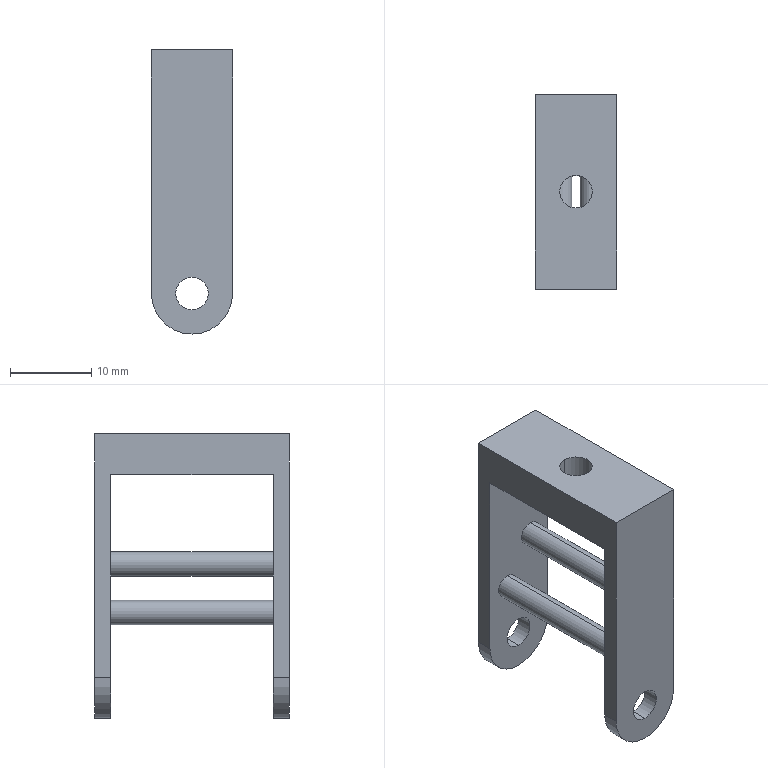Part | SolidWorks | features ICE 4, Extrusion 1 | 1 solid | 22 faces | box 10 x 24 x 35 mm | volume 2527 mm3 | cylinder 14 | plane 8 | commonest cylinder face diameters 4 x6 3 x4 10 x4
STEP:
#1=CARTESIAN_POINT('',(2.,2.,15.5));
#2=VERTEX_POINT('',#1);
#3=CARTESIAN_POINT('',(2.,2.,12.5));
#4=VERTEX_POINT('',#3);
#5=CARTESIAN_POINT('',(2.,2.,14.));
#6=DIRECTION('',(0.,1.,0.));
#7=DIRECTION('',(0.,0.,-1.));
#8=AXIS2_PLACEMENT_3D('',#5,#6,#7);
#9=CIRCLE('',#8,1.5);
#10=EDGE_CURVE('',#2,#4,#9,.T.);
#11=ORIENTED_EDGE('',*,*,#10,.T.);
#12=CARTESIAN_POINT('',(2.,22.,12.5));
#13=VERTEX_POINT('',#12);
#14=CARTESIAN_POINT('',(2.,-2.243,12.5));
#15=DIRECTION('',(0.,1.,0.));
#16=VECTOR('',#15,1000.);
#17=LINE('',#14,#16);
#18=EDGE_CURVE('',#4,#13,#17,.T.);
#19=ORIENTED_EDGE('',*,*,#18,.T.);
#20=CARTESIAN_POINT('',(2.,22.,15.5));
#21=VERTEX_POINT('',#20);
#22=CARTESIAN_POINT('',(2.,22.,14.));
#23=DIRECTION('',(0.,1.,0.));
#24=DIRECTION('',(0.,0.,1.));
#25=AXIS2_PLACEMENT_3D('',#22,#23,#24);
#26=CIRCLE('',#25,1.5);
#27=EDGE_CURVE('',#21,#13,#26,.T.);
#28=ORIENTED_EDGE('',*,*,#27,.F.);
#29=CARTESIAN_POINT('',(2.,-2.243,15.5));
#30=DIRECTION('',(0.,1.,0.));
#31=VECTOR('',#30,1000.);
#32=LINE('',#29,#31);
#33=EDGE_CURVE('',#2,#21,#32,.T.);
#34=ORIENTED_EDGE('',*,*,#33,.F.);
#35=EDGE_LOOP('',(#11,#19,#28,#34));
#36=FACE_OUTER_BOUND('',#35,.T.);
#37=CARTESIAN_POINT('',(2.,-2.243,14.));
#38=DIRECTION('',(0.,1.,0.));
#39=DIRECTION('',(0.,0.,1.));
#40=AXIS2_PLACEMENT_3D('',#37,#38,#39);
#41=CYLINDRICAL_SURFACE('',#40,1.5);
#42=ADVANCED_FACE('',(#36),#41,.T.);
#43=CARTESIAN_POINT('',(-2.,2.,9.5));
#44=VERTEX_POINT('',#43);
#45=CARTESIAN_POINT('',(-2.,2.,6.5));
#46=VERTEX_POINT('',#45);
#47=CARTESIAN_POINT('',(-2.,2.,8.));
#48=DIRECTION('',(0.,1.,0.));
#49=DIRECTION('',(0.,0.,-1.));
#50=AXIS2_PLACEMENT_3D('',#47,#48,#49);
#51=CIRCLE('',#50,1.5);
#52=EDGE_CURVE('',#44,#46,#51,.T.);
#53=ORIENTED_EDGE('',*,*,#52,.T.);
#54=CARTESIAN_POINT('',(-2.,22.,6.5));
#55=VERTEX_POINT('',#54);
#56=CARTESIAN_POINT('',(-2.,-2.243,6.5));
#57=DIRECTION('',(0.,1.,0.));
#58=VECTOR('',#57,1000.);
#59=LINE('',#56,#58);
#60=EDGE_CURVE('',#46,#55,#59,.T.);
#61=ORIENTED_EDGE('',*,*,#60,.T.);
#62=CARTESIAN_POINT('',(-2.,22.,9.5));
#63=VERTEX_POINT('',#62);
#64=CARTESIAN_POINT('',(-2.,22.,8.));
#65=DIRECTION('',(0.,1.,0.));
#66=DIRECTION('',(0.,0.,1.));
#67=AXIS2_PLACEMENT_3D('',#64,#65,#66);
#68=CIRCLE('',#67,1.5);
#69=EDGE_CURVE('',#63,#55,#68,.T.);
#70=ORIENTED_EDGE('',*,*,#69,.F.);
#71=CARTESIAN_POINT('',(-2.,-2.243,9.5));
#72=DIRECTION('',(0.,1.,0.));
#73=VECTOR('',#72,1000.);
#74=LINE('',#71,#73);
#75=EDGE_CURVE('',#44,#63,#74,.T.);
#76=ORIENTED_EDGE('',*,*,#75,.F.);
#77=EDGE_LOOP('',(#53,#61,#70,#76));
#78=FACE_OUTER_BOUND('',#77,.T.);
#79=CARTESIAN_POINT('',(-2.,-2.243,8.));
#80=DIRECTION('',(0.,1.,0.));
#81=DIRECTION('',(0.,0.,1.));
#82=AXIS2_PLACEMENT_3D('',#79,#80,#81);
#83=CYLINDRICAL_SURFACE('',#82,1.5);
#84=ADVANCED_FACE('',(#78),#83,.T.);
#85=CARTESIAN_POINT('',(0.,10.,30.));
#86=VERTEX_POINT('',#85);
#87=CARTESIAN_POINT('',(0.,14.,30.));
#88=VERTEX_POINT('',#87);
#89=CARTESIAN_POINT('',(0.,12.,30.));
#90=DIRECTION('',(0.,0.,-1.));
#91=DIRECTION('',(0.,1.,0.));
#92=AXIS2_PLACEMENT_3D('',#89,#90,#91);
#93=CIRCLE('',#92,2.);
#94=EDGE_CURVE('',#86,#88,#93,.T.);
#95=ORIENTED_EDGE('',*,*,#94,.F.);
#96=CARTESIAN_POINT('',(0.,10.,25.));
#97=VERTEX_POINT('',#96);
#98=CARTESIAN_POINT('',(0.,10.,30.));
#99=DIRECTION('',(0.,0.,-1.));
#100=VECTOR('',#99,1000.);
#101=LINE('',#98,#100);
#102=EDGE_CURVE('',#86,#97,#101,.T.);
#103=ORIENTED_EDGE('',*,*,#102,.T.);
#104=CARTESIAN_POINT('',(0.,14.,25.));
#105=VERTEX_POINT('',#104);
#106=CARTESIAN_POINT('',(0.,12.,25.));
#107=DIRECTION('',(0.,0.,-1.));
#108=DIRECTION('',(0.,1.,0.));
#109=AXIS2_PLACEMENT_3D('',#106,#107,#108);
#110=CIRCLE('',#109,2.);
#111=EDGE_CURVE('',#97,#105,#110,.T.);
#112=ORIENTED_EDGE('',*,*,#111,.T.);
#113=CARTESIAN_POINT('',(0.,14.,30.));
#114=DIRECTION('',(0.,0.,-1.));
#115=VECTOR('',#114,1000.);
#116=LINE('',#113,#115);
#117=EDGE_CURVE('',#88,#105,#116,.T.);
#118=ORIENTED_EDGE('',*,*,#117,.F.);
#119=EDGE_LOOP('',(#95,#103,#112,#118));
#120=FACE_OUTER_BOUND('',#119,.T.);
#121=CARTESIAN_POINT('',(0.,12.,30.));
#122=DIRECTION('',(0.,0.,-1.));
#123=DIRECTION('',(0.,1.,0.));
#124=AXIS2_PLACEMENT_3D('',#121,#122,#123);
#125=CYLINDRICAL_SURFACE('',#124,2.);
#126=ADVANCED_FACE('',(#120),#125,.F.);
#127=CARTESIAN_POINT('',(0.,0.,-2.));
#128=VERTEX_POINT('',#127);
#129=CARTESIAN_POINT('',(0.,0.,2.));
#130=VERTEX_POINT('',#129);
#131=CARTESIAN_POINT('',(0.,0.,0.));
#132=DIRECTION('',(0.,1.,0.));
#133=DIRECTION('',(0.,0.,1.));
#134=AXIS2_PLACEMENT_3D('',#131,#132,#133);
#135=CIRCLE('',#134,2.);
#136=EDGE_CURVE('',#128,#130,#135,.T.);
#137=ORIENTED_EDGE('',*,*,#136,.F.);
#138=CARTESIAN_POINT('',(0.,2.,-2.));
#139=VERTEX_POINT('',#138);
#140=CARTESIAN_POINT('',(0.,0.,-2.));
#141=DIRECTION('',(0.,1.,0.));
#142=VECTOR('',#141,1000.);
#143=LINE('',#140,#142);
#144=EDGE_CURVE('',#128,#139,#143,.T.);
#145=ORIENTED_EDGE('',*,*,#144,.T.);
#146=CARTESIAN_POINT('',(0.,2.,2.));
#147=VERTEX_POINT('',#146);
#148=CARTESIAN_POINT('',(0.,2.,0.));
#149=DIRECTION('',(0.,1.,0.));
#150=DIRECTION('',(0.,0.,-1.));
#151=AXIS2_PLACEMENT_3D('',#148,#149,#150);
#152=CIRCLE('',#151,2.);
#153=EDGE_CURVE('',#139,#147,#152,.T.);
#154=ORIENTED_EDGE('',*,*,#153,.T.);
#155=CARTESIAN_POINT('',(0.,0.,2.));
#156=DIRECTION('',(0.,1.,0.));
#157=VECTOR('',#156,1000.);
#158=LINE('',#155,#157);
#159=EDGE_CURVE('',#130,#147,#158,.T.);
#160=ORIENTED_EDGE('',*,*,#159,.F.);
#161=EDGE_LOOP('',(#137,#145,#154,#160));
#162=FACE_OUTER_BOUND('',#161,.T.);
#163=CARTESIAN_POINT('',(0.,0.,0.));
#164=DIRECTION('',(0.,1.,0.));
#165=DIRECTION('',(0.,0.,1.));
#166=AXIS2_PLACEMENT_3D('',#163,#164,#165);
#167=CYLINDRICAL_SURFACE('',#166,2.);
#168=ADVANCED_FACE('',(#162),#167,.F.);
#169=CARTESIAN_POINT('',(-5.,2.,0.));
#170=VERTEX_POINT('',#169);
#171=CARTESIAN_POINT('',(0.,2.,-5.));
#172=VERTEX_POINT('',#171);
#173=CARTESIAN_POINT('',(0.,2.,0.));
#174=DIRECTION('',(0.,-1.,0.));
#175=DIRECTION('',(0.,0.,-1.));
#176=AXIS2_PLACEMENT_3D('',#173,#174,#175);
#177=CIRCLE('',#176,5.);
#178=EDGE_CURVE('',#170,#172,#177,.T.);
#179=ORIENTED_EDGE('',*,*,#178,.T.);
#180=CARTESIAN_POINT('',(0.,0.,-5.));
#181=VERTEX_POINT('',#180);
#182=CARTESIAN_POINT('',(0.,24.,-5.));
#183=DIRECTION('',(0.,-1.,0.));
#184=VECTOR('',#183,1000.);
#185=LINE('',#182,#184);
#186=EDGE_CURVE('',#172,#181,#185,.T.);
#187=ORIENTED_EDGE('',*,*,#186,.T.);
#188=CARTESIAN_POINT('',(-5.,0.,0.));
#189=VERTEX_POINT('',#188);
#190=CARTESIAN_POINT('',(0.,0.,0.));
#191=DIRECTION('',(0.,1.,0.));
#192=DIRECTION('',(0.,0.,1.));
#193=AXIS2_PLACEMENT_3D('',#190,#191,#192);
#194=CIRCLE('',#193,5.);
#195=EDGE_CURVE('',#181,#189,#194,.T.);
#196=ORIENTED_EDGE('',*,*,#195,.T.);
#197=CARTESIAN_POINT('',(-5.,24.,0.));
#198=DIRECTION('',(0.,-1.,0.));
#199=VECTOR('',#198,1000.);
#200=LINE('',#197,#199);
#201=EDGE_CURVE('',#170,#189,#200,.T.);
#202=ORIENTED_EDGE('',*,*,#201,.F.);
#203=EDGE_LOOP('',(#179,#187,#196,#202));
#204=FACE_OUTER_BOUND('',#203,.T.);
#205=CARTESIAN_POINT('',(0.,24.,0.));
#206=DIRECTION('',(0.,-1.,0.));
#207=DIRECTION('',(0.,0.,-1.));
#208=AXIS2_PLACEMENT_3D('',#205,#206,#207);
#209=CYLINDRICAL_SURFACE('',#208,5.);
#210=ADVANCED_FACE('',(#204),#209,.T.);
#211=CARTESIAN_POINT('',(0.,22.,2.));
#212=VERTEX_POINT('',#211);
#213=CARTESIAN_POINT('',(0.,22.,-2.));
#214=VERTEX_POINT('',#213);
#215=CARTESIAN_POINT('',(0.,22.,0.));
#216=DIRECTION('',(0.,-1.,0.));
#217=DIRECTION('',(0.,0.,1.));
#218=AXIS2_PLACEMENT_3D('',#215,#216,#217);
#219=CIRCLE('',#218,2.);
#220=EDGE_CURVE('',#212,#214,#219,.T.);
#221=ORIENTED_EDGE('',*,*,#220,.T.);
#222=CARTESIAN_POINT('',(0.,24.,-2.));
#223=VERTEX_POINT('',#222);
#224=CARTESIAN_POINT('',(0.,0.,-2.));
#225=DIRECTION('',(0.,1.,0.));
#226=VECTOR('',#225,1000.);
#227=LINE('',#224,#226);
#228=EDGE_CURVE('',#214,#223,#227,.T.);
#229=ORIENTED_EDGE('',*,*,#228,.T.);
#230=CARTESIAN_POINT('',(0.,24.,2.));
#231=VERTEX_POINT('',#230);
#232=CARTESIAN_POINT('',(0.,24.,0.));
#233=DIRECTION('',(0.,1.,0.));
#234=DIRECTION('',(0.,0.,1.));
#235=AXIS2_PLACEMENT_3D('',#232,#233,#234);
#236=CIRCLE('',#235,2.);
#237=EDGE_CURVE('',#223,#231,#236,.T.);
#238=ORIENTED_EDGE('',*,*,#237,.T.);
#239=CARTESIAN_POINT('',(0.,0.,2.));
#240=DIRECTION('',(0.,1.,0.));
#241=VECTOR('',#240,1000.);
#242=LINE('',#239,#241);
#243=EDGE_CURVE('',#212,#231,#242,.T.);
#244=ORIENTED_EDGE('',*,*,#243,.F.);
#245=EDGE_LOOP('',(#221,#229,#238,#244));
#246=FACE_OUTER_BOUND('',#245,.T.);
#247=CARTESIAN_POINT('',(0.,0.,0.));
#248=DIRECTION('',(0.,1.,0.));
#249=DIRECTION('',(0.,0.,1.));
#250=AXIS2_PLACEMENT_3D('',#247,#248,#249);
#251=CYLINDRICAL_SURFACE('',#250,2.);
#252=ADVANCED_FACE('',(#246),#251,.F.);
#253=CARTESIAN_POINT('',(0.,24.,-5.));
#254=VERTEX_POINT('',#253);
#255=CARTESIAN_POINT('',(-5.,24.,0.));
#256=VERTEX_POINT('',#255);
#257=CARTESIAN_POINT('',(0.,24.,0.));
#258=DIRECTION('',(0.,1.,0.));
#259=DIRECTION('',(0.,0.,1.));
#260=AXIS2_PLACEMENT_3D('',#257,#258,#259);
#261=CIRCLE('',#260,5.);
#262=EDGE_CURVE('',#254,#256,#261,.T.);
#263=ORIENTED_EDGE('',*,*,#262,.F.);
#264=CARTESIAN_POINT('',(0.,22.,-5.));
#265=VERTEX_POINT('',#264);
#266=CARTESIAN_POINT('',(0.,24.,-5.));
#267=DIRECTION('',(0.,-1.,0.));
#268=VECTOR('',#267,1000.);
#269=LINE('',#266,#268);
#270=EDGE_CURVE('',#254,#265,#269,.T.);
#271=ORIENTED_EDGE('',*,*,#270,.T.);
#272=CARTESIAN_POINT('',(-5.,22.,0.));
#273=VERTEX_POINT('',#272);
#274=CARTESIAN_POINT('',(0.,22.,0.));
#275=DIRECTION('',(0.,1.,0.));
#276=DIRECTION('',(0.,0.,1.));
#277=AXIS2_PLACEMENT_3D('',#274,#275,#276);
#278=CIRCLE('',#277,5.);
#279=EDGE_CURVE('',#265,#273,#278,.T.);
#280=ORIENTED_EDGE('',*,*,#279,.T.);
#281=CARTESIAN_POINT('',(-5.,24.,0.));
#282=DIRECTION('',(0.,-1.,0.));
#283=VECTOR('',#282,1000.);
#284=LINE('',#281,#283);
#285=EDGE_CURVE('',#256,#273,#284,.T.);
#286=ORIENTED_EDGE('',*,*,#285,.F.);
#287=EDGE_LOOP('',(#263,#271,#280,#286));
#288=FACE_OUTER_BOUND('',#287,.T.);
#289=CARTESIAN_POINT('',(0.,24.,0.));
#290=DIRECTION('',(0.,-1.,0.));
#291=DIRECTION('',(0.,0.,-1.));
#292=AXIS2_PLACEMENT_3D('',#289,#290,#291);
#293=CYLINDRICAL_SURFACE('',#292,5.);
#294=ADVANCED_FACE('',(#288),#293,.T.);
#295=ORIENTED_EDGE('',*,*,#270,.F.);
#296=CARTESIAN_POINT('',(5.,24.,0.));
#297=VERTEX_POINT('',#296);
#298=CARTESIAN_POINT('',(0.,24.,0.));
#299=DIRECTION('',(0.,1.,0.));
#300=DIRECTION('',(0.,0.,1.));
#301=AXIS2_PLACEMENT_3D('',#298,#299,#300);
#302=CIRCLE('',#301,5.);
#303=EDGE_CURVE('',#297,#254,#302,.T.);
#304=ORIENTED_EDGE('',*,*,#303,.F.);
#305=CARTESIAN_POINT('',(5.,22.,0.));
#306=VERTEX_POINT('',#305);
#307=CARTESIAN_POINT('',(5.,24.,0.));
#308=DIRECTION('',(0.,-1.,0.));
#309=VECTOR('',#308,1000.);
#310=LINE('',#307,#309);
#311=EDGE_CURVE('',#297,#306,#310,.T.);
#312=ORIENTED_EDGE('',*,*,#311,.T.);
#313=CARTESIAN_POINT('',(0.,22.,0.));
#314=DIRECTION('',(0.,1.,0.));
#315=DIRECTION('',(0.,0.,1.));
#316=AXIS2_PLACEMENT_3D('',#313,#314,#315);
#317=CIRCLE('',#316,5.);
#318=EDGE_CURVE('',#306,#265,#317,.T.);
#319=ORIENTED_EDGE('',*,*,#318,.T.);
#320=EDGE_LOOP('',(#295,#304,#312,#319));
#321=FACE_OUTER_BOUND('',#320,.T.);
#322=CARTESIAN_POINT('',(0.,24.,0.));
#323=DIRECTION('',(0.,-1.,0.));
#324=DIRECTION('',(0.,0.,-1.));
#325=AXIS2_PLACEMENT_3D('',#322,#323,#324);
#326=CYLINDRICAL_SURFACE('',#325,5.);
#327=ADVANCED_FACE('',(#321),#326,.T.);
#328=ORIENTED_EDGE('',*,*,#228,.F.);
#329=CARTESIAN_POINT('',(0.,22.,0.));
#330=DIRECTION('',(0.,-1.,0.));
#331=DIRECTION('',(0.,0.,1.));
#332=AXIS2_PLACEMENT_3D('',#329,#330,#331);
#333=CIRCLE('',#332,2.);
#334=EDGE_CURVE('',#214,#212,#333,.T.);
#335=ORIENTED_EDGE('',*,*,#334,.T.);
#336=ORIENTED_EDGE('',*,*,#243,.T.);
#337=CARTESIAN_POINT('',(0.,24.,0.));
#338=DIRECTION('',(0.,1.,0.));
#339=DIRECTION('',(0.,0.,1.));
#340=AXIS2_PLACEMENT_3D('',#337,#338,#339);
#341=CIRCLE('',#340,2.);
#342=EDGE_CURVE('',#231,#223,#341,.T.);
#343=ORIENTED_EDGE('',*,*,#342,.T.);
#344=EDGE_LOOP('',(#328,#335,#336,#343));
#345=FACE_OUTER_BOUND('',#344,.T.);
#346=CARTESIAN_POINT('',(0.,0.,0.));
#347=DIRECTION('',(0.,1.,0.));
#348=DIRECTION('',(0.,0.,1.));
#349=AXIS2_PLACEMENT_3D('',#346,#347,#348);
#350=CYLINDRICAL_SURFACE('',#349,2.);
#351=ADVANCED_FACE('',(#345),#350,.F.);
#352=ORIENTED_EDGE('',*,*,#186,.F.);
#353=CARTESIAN_POINT('',(5.,2.,0.));
#354=VERTEX_POINT('',#353);
#355=CARTESIAN_POINT('',(0.,2.,0.));
#356=DIRECTION('',(0.,-1.,0.));
#357=DIRECTION('',(0.,0.,-1.));
#358=AXIS2_PLACEMENT_3D('',#355,#356,#357);
#359=CIRCLE('',#358,5.);
#360=EDGE_CURVE('',#172,#354,#359,.T.);
#361=ORIENTED_EDGE('',*,*,#360,.T.);
#362=CARTESIAN_POINT('',(5.,0.,0.));
#363=VERTEX_POINT('',#362);
#364=CARTESIAN_POINT('',(5.,24.,0.));
#365=DIRECTION('',(0.,-1.,0.));
#366=VECTOR('',#365,1000.);
#367=LINE('',#364,#366);
#368=EDGE_CURVE('',#354,#363,#367,.T.);
#369=ORIENTED_EDGE('',*,*,#368,.T.);
#370=CARTESIAN_POINT('',(0.,0.,0.));
#371=DIRECTION('',(0.,1.,0.));
#372=DIRECTION('',(0.,0.,1.));
#373=AXIS2_PLACEMENT_3D('',#370,#371,#372);
#374=CIRCLE('',#373,5.);
#375=EDGE_CURVE('',#363,#181,#374,.T.);
#376=ORIENTED_EDGE('',*,*,#375,.T.);
#377=EDGE_LOOP('',(#352,#361,#369,#376));
#378=FACE_OUTER_BOUND('',#377,.T.);
#379=CARTESIAN_POINT('',(0.,24.,0.));
#380=DIRECTION('',(0.,-1.,0.));
#381=DIRECTION('',(0.,0.,-1.));
#382=AXIS2_PLACEMENT_3D('',#379,#380,#381);
#383=CYLINDRICAL_SURFACE('',#382,5.);
#384=ADVANCED_FACE('',(#378),#383,.T.);
#385=ORIENTED_EDGE('',*,*,#285,.T.);
#386=CARTESIAN_POINT('',(-5.,22.,25.));
#387=VERTEX_POINT('',#386);
#388=CARTESIAN_POINT('',(-5.,22.,-7.589));
#389=DIRECTION('',(0.,0.,1.));
#390=VECTOR('',#389,1000.);
#391=LINE('',#388,#390);
#392=EDGE_CURVE('',#273,#387,#391,.T.);
#393=ORIENTED_EDGE('',*,*,#392,.T.);
#394=CARTESIAN_POINT('',(-5.,2.,25.));
#395=VERTEX_POINT('',#394);
#396=CARTESIAN_POINT('',(-5.,22.,25.));
#397=DIRECTION('',(0.,-1.,0.));
#398=VECTOR('',#397,1000.);
#399=LINE('',#396,#398);
#400=EDGE_CURVE('',#387,#395,#399,.T.);
#401=ORIENTED_EDGE('',*,*,#400,.T.);
#402=CARTESIAN_POINT('',(-5.,2.,25.));
#403=DIRECTION('',(0.,0.,-1.));
#404=VECTOR('',#403,1000.);
#405=LINE('',#402,#404);
#406=EDGE_CURVE('',#395,#170,#405,.T.);
#407=ORIENTED_EDGE('',*,*,#406,.T.);
#408=ORIENTED_EDGE('',*,*,#201,.T.);
#409=CARTESIAN_POINT('',(-5.,0.,30.));
#410=VERTEX_POINT('',#409);
#411=CARTESIAN_POINT('',(-5.,0.,0.));
#412=DIRECTION('',(0.,0.,1.));
#413=VECTOR('',#412,1000.);
#414=LINE('',#411,#413);
#415=EDGE_CURVE('',#189,#410,#414,.T.);
#416=ORIENTED_EDGE('',*,*,#415,.T.);
#417=CARTESIAN_POINT('',(-5.,24.,30.));
#418=VERTEX_POINT('',#417);
#419=CARTESIAN_POINT('',(-5.,24.,30.));
#420=DIRECTION('',(0.,-1.,0.));
#421=VECTOR('',#420,1000.);
#422=LINE('',#419,#421);
#423=EDGE_CURVE('',#418,#410,#422,.T.);
#424=ORIENTED_EDGE('',*,*,#423,.F.);
#425=CARTESIAN_POINT('',(-5.,24.,0.));
#426=DIRECTION('',(0.,0.,1.));
#427=VECTOR('',#426,1000.);
#428=LINE('',#425,#427);
#429=EDGE_CURVE('',#256,#418,#428,.T.);
#430=ORIENTED_EDGE('',*,*,#429,.F.);
#431=EDGE_LOOP('',(#385,#393,#401,#407,#408,#416,#424,#430));
#432=FACE_OUTER_BOUND('',#431,.T.);
#433=CARTESIAN_POINT('',(-5.,24.,0.));
#434=DIRECTION('',(1.,0.,0.));
#435=DIRECTION('',(0.,0.,-1.));
#436=AXIS2_PLACEMENT_3D('',#433,#434,#435);
#437=PLANE('',#436);
#438=ADVANCED_FACE('',(#432),#437,.F.);
#439=CARTESIAN_POINT('',(0.,12.,30.));
#440=DIRECTION('',(0.,0.,-1.));
#441=DIRECTION('',(0.,1.,0.));
#442=AXIS2_PLACEMENT_3D('',#439,#440,#441);
#443=CIRCLE('',#442,2.);
#444=EDGE_CURVE('',#88,#86,#443,.T.);
#445=ORIENTED_EDGE('',*,*,#444,.T.);
#446=ORIENTED_EDGE('',*,*,#94,.T.);
#447=EDGE_LOOP('',(#445,#446));
#448=FACE_BOUND('',#447,.T.);
#449=CARTESIAN_POINT('',(5.,0.,30.));
#450=VERTEX_POINT('',#449);
#451=CARTESIAN_POINT('',(-5.,0.,30.));
#452=DIRECTION('',(1.,0.,0.));
#453=VECTOR('',#452,1000.);
#454=LINE('',#451,#453);
#455=EDGE_CURVE('',#410,#450,#454,.T.);
#456=ORIENTED_EDGE('',*,*,#455,.T.);
#457=CARTESIAN_POINT('',(5.,24.,30.));
#458=VERTEX_POINT('',#457);
#459=CARTESIAN_POINT('',(5.,24.,30.));
#460=DIRECTION('',(0.,-1.,0.));
#461=VECTOR('',#460,1000.);
#462=LINE('',#459,#461);
#463=EDGE_CURVE('',#458,#450,#462,.T.);
#464=ORIENTED_EDGE('',*,*,#463,.F.);
#465=CARTESIAN_POINT('',(-5.,24.,30.));
#466=DIRECTION('',(1.,0.,0.));
#467=VECTOR('',#466,1000.);
#468=LINE('',#465,#467);
#469=EDGE_CURVE('',#418,#458,#468,.T.);
#470=ORIENTED_EDGE('',*,*,#469,.F.);
#471=ORIENTED_EDGE('',*,*,#423,.T.);
#472=EDGE_LOOP('',(#456,#464,#470,#471));
#473=FACE_OUTER_BOUND('',#472,.T.);
#474=CARTESIAN_POINT('',(-5.,24.,30.));
#475=DIRECTION('',(0.,0.,-1.));
#476=DIRECTION('',(-1.,0.,0.));
#477=AXIS2_PLACEMENT_3D('',#474,#475,#476);
#478=PLANE('',#477);
#479=ADVANCED_FACE('',(#448,#473),#478,.F.);
#480=CARTESIAN_POINT('',(5.,22.,25.));
#481=VERTEX_POINT('',#480);
#482=CARTESIAN_POINT('',(5.,2.,25.));
#483=VERTEX_POINT('',#482);
#484=CARTESIAN_POINT('',(5.,22.,25.));
#485=DIRECTION('',(0.,-1.,0.));
#486=VECTOR('',#485,1000.);
#487=LINE('',#484,#486);
#488=EDGE_CURVE('',#481,#483,#487,.T.);
#489=ORIENTED_EDGE('',*,*,#488,.F.);
#490=CARTESIAN_POINT('',(5.,22.,-7.589));
#491=DIRECTION('',(0.,0.,1.));
#492=VECTOR('',#491,1000.);
#493=LINE('',#490,#492);
#494=EDGE_CURVE('',#306,#481,#493,.T.);
#495=ORIENTED_EDGE('',*,*,#494,.F.);
#496=ORIENTED_EDGE('',*,*,#311,.F.);
#497=CARTESIAN_POINT('',(5.,24.,0.));
#498=DIRECTION('',(0.,0.,-1.));
#499=VECTOR('',#498,1000.);
#500=LINE('',#497,#499);
#501=EDGE_CURVE('',#458,#297,#500,.T.);
#502=ORIENTED_EDGE('',*,*,#501,.F.);
#503=ORIENTED_EDGE('',*,*,#463,.T.);
#504=CARTESIAN_POINT('',(5.,0.,0.));
#505=DIRECTION('',(0.,0.,-1.));
#506=VECTOR('',#505,1000.);
#507=LINE('',#504,#506);
#508=EDGE_CURVE('',#450,#363,#507,.T.);
#509=ORIENTED_EDGE('',*,*,#508,.T.);
#510=ORIENTED_EDGE('',*,*,#368,.F.);
#511=CARTESIAN_POINT('',(5.,2.,25.));
#512=DIRECTION('',(0.,0.,-1.));
#513=VECTOR('',#512,1000.);
#514=LINE('',#511,#513);
#515=EDGE_CURVE('',#483,#354,#514,.T.);
#516=ORIENTED_EDGE('',*,*,#515,.F.);
#517=EDGE_LOOP('',(#489,#495,#496,#502,#503,#509,#510,#516));
#518=FACE_OUTER_BOUND('',#517,.T.);
#519=CARTESIAN_POINT('',(5.,24.,0.));
#520=DIRECTION('',(-1.,0.,0.));
#521=DIRECTION('',(0.,0.,1.));
#522=AXIS2_PLACEMENT_3D('',#519,#520,#521);
#523=PLANE('',#522);
#524=ADVANCED_FACE('',(#518),#523,.F.);
#525=ORIENTED_EDGE('',*,*,#342,.F.);
#526=ORIENTED_EDGE('',*,*,#237,.F.);
#527=EDGE_LOOP('',(#525,#526));
#528=FACE_BOUND('',#527,.T.);
#529=ORIENTED_EDGE('',*,*,#303,.T.);
#530=ORIENTED_EDGE('',*,*,#262,.T.);
#531=ORIENTED_EDGE('',*,*,#429,.T.);
#532=ORIENTED_EDGE('',*,*,#469,.T.);
#533=ORIENTED_EDGE('',*,*,#501,.T.);
#534=EDGE_LOOP('',(#529,#530,#531,#532,#533));
#535=FACE_OUTER_BOUND('',#534,.T.);
#536=CARTESIAN_POINT('',(0.,24.,0.));
#537=DIRECTION('',(0.,1.,0.));
#538=DIRECTION('',(0.,0.,1.));
#539=AXIS2_PLACEMENT_3D('',#536,#537,#538);
#540=PLANE('',#539);
#541=ADVANCED_FACE('',(#528,#535),#540,.T.);
#542=CARTESIAN_POINT('',(0.,0.,0.));
#543=DIRECTION('',(0.,1.,0.));
#544=DIRECTION('',(0.,0.,1.));
#545=AXIS2_PLACEMENT_3D('',#542,#543,#544);
#546=CIRCLE('',#545,2.);
#547=EDGE_CURVE('',#130,#128,#546,.T.);
#548=ORIENTED_EDGE('',*,*,#547,.T.);
#549=ORIENTED_EDGE('',*,*,#136,.T.);
#550=EDGE_LOOP('',(#548,#549));
#551=FACE_BOUND('',#550,.T.);
#552=ORIENTED_EDGE('',*,*,#375,.F.);
#553=ORIENTED_EDGE('',*,*,#508,.F.);
#554=ORIENTED_EDGE('',*,*,#455,.F.);
#555=ORIENTED_EDGE('',*,*,#415,.F.);
#556=ORIENTED_EDGE('',*,*,#195,.F.);
#557=EDGE_LOOP('',(#552,#553,#554,#555,#556));
#558=FACE_OUTER_BOUND('',#557,.T.);
#559=CARTESIAN_POINT('',(0.,0.,0.));
#560=DIRECTION('',(0.,1.,0.));
#561=DIRECTION('',(0.,0.,1.));
#562=AXIS2_PLACEMENT_3D('',#559,#560,#561);
#563=PLANE('',#562);
#564=ADVANCED_FACE('',(#551,#558),#563,.F.);
#565=ORIENTED_EDGE('',*,*,#144,.F.);
#566=ORIENTED_EDGE('',*,*,#547,.F.);
#567=ORIENTED_EDGE('',*,*,#159,.T.);
#568=CARTESIAN_POINT('',(0.,2.,0.));
#569=DIRECTION('',(0.,1.,0.));
#570=DIRECTION('',(0.,0.,-1.));
#571=AXIS2_PLACEMENT_3D('',#568,#569,#570);
#572=CIRCLE('',#571,2.);
#573=EDGE_CURVE('',#147,#139,#572,.T.);
#574=ORIENTED_EDGE('',*,*,#573,.T.);
#575=EDGE_LOOP('',(#565,#566,#567,#574));
#576=FACE_OUTER_BOUND('',#575,.T.);
#577=CARTESIAN_POINT('',(0.,0.,0.));
#578=DIRECTION('',(0.,1.,0.));
#579=DIRECTION('',(0.,0.,1.));
#580=AXIS2_PLACEMENT_3D('',#577,#578,#579);
#581=CYLINDRICAL_SURFACE('',#580,2.);
#582=ADVANCED_FACE('',(#576),#581,.F.);
#583=ORIENTED_EDGE('',*,*,#27,.T.);
#584=CARTESIAN_POINT('',(2.,22.,14.));
#585=DIRECTION('',(0.,1.,0.));
#586=DIRECTION('',(0.,0.,1.));
#587=AXIS2_PLACEMENT_3D('',#584,#585,#586);
#588=CIRCLE('',#587,1.5);
#589=EDGE_CURVE('',#13,#21,#588,.T.);
#590=ORIENTED_EDGE('',*,*,#589,.T.);
#591=EDGE_LOOP('',(#583,#590));
#592=FACE_BOUND('',#591,.T.);
#593=ORIENTED_EDGE('',*,*,#69,.T.);
#594=CARTESIAN_POINT('',(-2.,22.,8.));
#595=DIRECTION('',(0.,1.,0.));
#596=DIRECTION('',(0.,0.,1.));
#597=AXIS2_PLACEMENT_3D('',#594,#595,#596);
#598=CIRCLE('',#597,1.5);
#599=EDGE_CURVE('',#55,#63,#598,.T.);
#600=ORIENTED_EDGE('',*,*,#599,.T.);
#601=EDGE_LOOP('',(#593,#600));
#602=FACE_BOUND('',#601,.T.);
#603=ORIENTED_EDGE('',*,*,#220,.F.);
#604=ORIENTED_EDGE('',*,*,#334,.F.);
#605=EDGE_LOOP('',(#603,#604));
#606=FACE_BOUND('',#605,.T.);
#607=ORIENTED_EDGE('',*,*,#494,.T.);
#608=CARTESIAN_POINT('',(-5.,22.,25.));
#609=DIRECTION('',(1.,0.,0.));
#610=VECTOR('',#609,1000.);
#611=LINE('',#608,#610);
#612=EDGE_CURVE('',#387,#481,#611,.T.);
#613=ORIENTED_EDGE('',*,*,#612,.F.);
#614=ORIENTED_EDGE('',*,*,#392,.F.);
#615=ORIENTED_EDGE('',*,*,#279,.F.);
#616=ORIENTED_EDGE('',*,*,#318,.F.);
#617=EDGE_LOOP('',(#607,#613,#614,#615,#616));
#618=FACE_OUTER_BOUND('',#617,.T.);
#619=CARTESIAN_POINT('',(-5.,22.,-7.589));
#620=DIRECTION('',(0.,1.,0.));
#621=DIRECTION('',(0.,0.,1.));
#622=AXIS2_PLACEMENT_3D('',#619,#620,#621);
#623=PLANE('',#622);
#624=ADVANCED_FACE('',(#592,#602,#606,#618),#623,.F.);
#625=ORIENTED_EDGE('',*,*,#10,.F.);
#626=CARTESIAN_POINT('',(2.,2.,14.));
#627=DIRECTION('',(0.,1.,0.));
#628=DIRECTION('',(0.,0.,-1.));
#629=AXIS2_PLACEMENT_3D('',#626,#627,#628);
#630=CIRCLE('',#629,1.5);
#631=EDGE_CURVE('',#4,#2,#630,.T.);
#632=ORIENTED_EDGE('',*,*,#631,.F.);
#633=EDGE_LOOP('',(#625,#632));
#634=FACE_BOUND('',#633,.T.);
#635=ORIENTED_EDGE('',*,*,#52,.F.);
#636=CARTESIAN_POINT('',(-2.,2.,8.));
#637=DIRECTION('',(0.,1.,0.));
#638=DIRECTION('',(0.,0.,-1.));
#639=AXIS2_PLACEMENT_3D('',#636,#637,#638);
#640=CIRCLE('',#639,1.5);
#641=EDGE_CURVE('',#46,#44,#640,.T.);
#642=ORIENTED_EDGE('',*,*,#641,.F.);
#643=EDGE_LOOP('',(#635,#642));
#644=FACE_BOUND('',#643,.T.);
#645=ORIENTED_EDGE('',*,*,#573,.F.);
#646=ORIENTED_EDGE('',*,*,#153,.F.);
#647=EDGE_LOOP('',(#645,#646));
#648=FACE_BOUND('',#647,.T.);
#649=ORIENTED_EDGE('',*,*,#406,.F.);
#650=CARTESIAN_POINT('',(-5.,2.,25.));
#651=DIRECTION('',(1.,0.,0.));
#652=VECTOR('',#651,1000.);
#653=LINE('',#650,#652);
#654=EDGE_CURVE('',#395,#483,#653,.T.);
#655=ORIENTED_EDGE('',*,*,#654,.T.);
#656=ORIENTED_EDGE('',*,*,#515,.T.);
#657=ORIENTED_EDGE('',*,*,#360,.F.);
#658=ORIENTED_EDGE('',*,*,#178,.F.);
#659=EDGE_LOOP('',(#649,#655,#656,#657,#658));
#660=FACE_OUTER_BOUND('',#659,.T.);
#661=CARTESIAN_POINT('',(-5.,2.,25.));
#662=DIRECTION('',(0.,-1.,0.));
#663=DIRECTION('',(0.,0.,-1.));
#664=AXIS2_PLACEMENT_3D('',#661,#662,#663);
#665=PLANE('',#664);
#666=ADVANCED_FACE('',(#634,#644,#648,#660),#665,.F.);
#667=CARTESIAN_POINT('',(0.,12.,25.));
#668=DIRECTION('',(0.,0.,-1.));
#669=DIRECTION('',(0.,1.,0.));
#670=AXIS2_PLACEMENT_3D('',#667,#668,#669);
#671=CIRCLE('',#670,2.);
#672=EDGE_CURVE('',#105,#97,#671,.T.);
#673=ORIENTED_EDGE('',*,*,#672,.F.);
#674=ORIENTED_EDGE('',*,*,#111,.F.);
#675=EDGE_LOOP('',(#673,#674));
#676=FACE_BOUND('',#675,.T.);
#677=ORIENTED_EDGE('',*,*,#654,.F.);
#678=ORIENTED_EDGE('',*,*,#400,.F.);
#679=ORIENTED_EDGE('',*,*,#612,.T.);
#680=ORIENTED_EDGE('',*,*,#488,.T.);
#681=EDGE_LOOP('',(#677,#678,#679,#680));
#682=FACE_OUTER_BOUND('',#681,.T.);
#683=CARTESIAN_POINT('',(-5.,22.,25.));
#684=DIRECTION('',(0.,0.,1.));
#685=DIRECTION('',(0.,-1.,0.));
#686=AXIS2_PLACEMENT_3D('',#683,#684,#685);
#687=PLANE('',#686);
#688=ADVANCED_FACE('',(#676,#682),#687,.F.);
#689=ORIENTED_EDGE('',*,*,#102,.F.);
#690=ORIENTED_EDGE('',*,*,#444,.F.);
#691=ORIENTED_EDGE('',*,*,#117,.T.);
#692=ORIENTED_EDGE('',*,*,#672,.T.);
#693=EDGE_LOOP('',(#689,#690,#691,#692));
#694=FACE_OUTER_BOUND('',#693,.T.);
#695=CARTESIAN_POINT('',(0.,12.,30.));
#696=DIRECTION('',(0.,0.,-1.));
#697=DIRECTION('',(0.,1.,0.));
#698=AXIS2_PLACEMENT_3D('',#695,#696,#697);
#699=CYLINDRICAL_SURFACE('',#698,2.);
#700=ADVANCED_FACE('',(#694),#699,.F.);
#701=ORIENTED_EDGE('',*,*,#60,.F.);
#702=ORIENTED_EDGE('',*,*,#641,.T.);
#703=ORIENTED_EDGE('',*,*,#75,.T.);
#704=ORIENTED_EDGE('',*,*,#599,.F.);
#705=EDGE_LOOP('',(#701,#702,#703,#704));
#706=FACE_OUTER_BOUND('',#705,.T.);
#707=CARTESIAN_POINT('',(-2.,-2.243,8.));
#708=DIRECTION('',(0.,1.,0.));
#709=DIRECTION('',(0.,0.,1.));
#710=AXIS2_PLACEMENT_3D('',#707,#708,#709);
#711=CYLINDRICAL_SURFACE('',#710,1.5);
#712=ADVANCED_FACE('',(#706),#711,.T.);
#713=ORIENTED_EDGE('',*,*,#18,.F.);
#714=ORIENTED_EDGE('',*,*,#631,.T.);
#715=ORIENTED_EDGE('',*,*,#33,.T.);
#716=ORIENTED_EDGE('',*,*,#589,.F.);
#717=EDGE_LOOP('',(#713,#714,#715,#716));
#718=FACE_OUTER_BOUND('',#717,.T.);
#719=CARTESIAN_POINT('',(2.,-2.243,14.));
#720=DIRECTION('',(0.,1.,0.));
#721=DIRECTION('',(0.,0.,1.));
#722=AXIS2_PLACEMENT_3D('',#719,#720,#721);
#723=CYLINDRICAL_SURFACE('',#722,1.5);
#724=ADVANCED_FACE('',(#718),#723,.T.);
#725=CLOSED_SHELL('',(#42,#84,#126,#168,#210,#252,#294,#327,#351,#384,#438,#479,#524,#541,#564,#582,#624,#666,#688,#700,#712,#724));
#726=MANIFOLD_SOLID_BREP('',#725);
#727=CARTESIAN_POINT('',(0.,0.,0.));
#728=DIRECTION('',(0.,0.,1.));
#729=DIRECTION('',(1.,0.,0.));
#730=AXIS2_PLACEMENT_3D('',#727,#728,#729);
#731=(LENGTH_UNIT()NAMED_UNIT(*)SI_UNIT(.MILLI.,.METRE.));
#732=UNCERTAINTY_MEASURE_WITH_UNIT(LENGTH_MEASURE(0.00001),#731,'','');
#733=(NAMED_UNIT(*)PLANE_ANGLE_UNIT()SI_UNIT($,.RADIAN.));
#734=(NAMED_UNIT(*)SI_UNIT($,.STERADIAN.)SOLID_ANGLE_UNIT());
#735=(GEOMETRIC_REPRESENTATION_CONTEXT(3)GLOBAL_UNCERTAINTY_ASSIGNED_CONTEXT((#732))GLOBAL_UNIT_ASSIGNED_CONTEXT((#731,#733,#734))REPRESENTATION_CONTEXT('',''));
#736=ADVANCED_BREP_SHAPE_REPRESENTATION('',(#726,#730),#735);